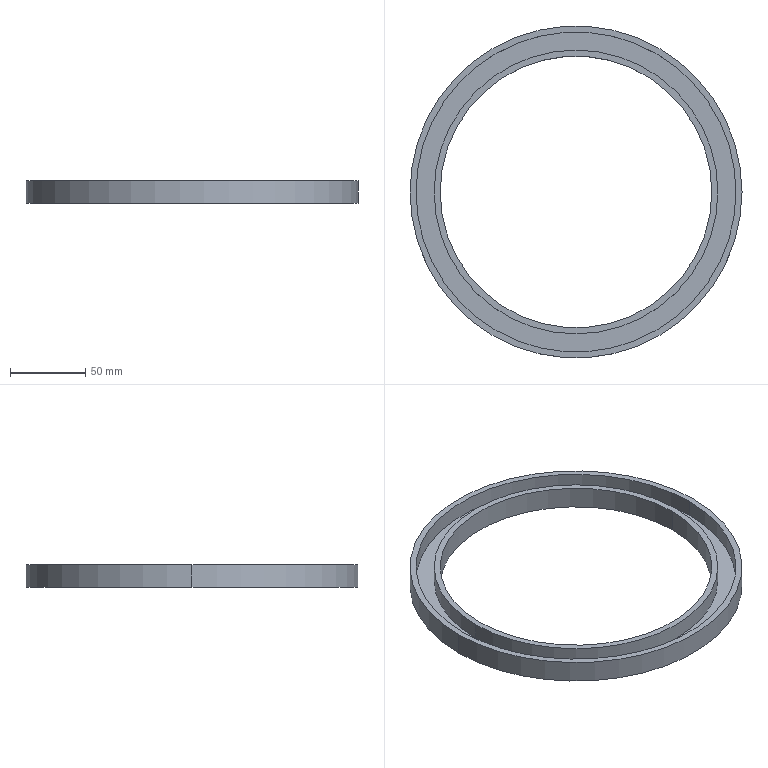Part | SolidWorks | features Extrusion 1, Shell 1 | 1 solid | 12 faces | box 220 x 220 x 15 mm | volume 105558 mm3 | cylinder 8 | plane 4 | commonest cylinder face diameters 180 x2 188 x2 212 x2 220 x2
STEP:
#1=CARTESIAN_POINT('',(94.,0.,15.));
#2=VERTEX_POINT('',#1);
#3=CARTESIAN_POINT('',(-94.,0.,15.));
#4=VERTEX_POINT('',#3);
#5=CARTESIAN_POINT('',(0.,0.,15.));
#6=DIRECTION('',(0.,0.,1.));
#7=DIRECTION('',(1.,0.,0.));
#8=AXIS2_PLACEMENT_3D('',#5,#6,#7);
#9=CIRCLE('',#8,94.);
#10=EDGE_CURVE('',#2,#4,#9,.T.);
#11=ORIENTED_EDGE('',*,*,#10,.F.);
#12=CARTESIAN_POINT('',(94.,0.,4.));
#13=VERTEX_POINT('',#12);
#14=CARTESIAN_POINT('',(94.,0.,15.));
#15=DIRECTION('',(0.,0.,-1.));
#16=VECTOR('',#15,1000.);
#17=LINE('',#14,#16);
#18=EDGE_CURVE('',#2,#13,#17,.T.);
#19=ORIENTED_EDGE('',*,*,#18,.T.);
#20=CARTESIAN_POINT('',(-94.,0.,4.));
#21=VERTEX_POINT('',#20);
#22=CARTESIAN_POINT('',(0.,0.,4.));
#23=DIRECTION('',(0.,0.,1.));
#24=DIRECTION('',(1.,0.,0.));
#25=AXIS2_PLACEMENT_3D('',#22,#23,#24);
#26=CIRCLE('',#25,94.);
#27=EDGE_CURVE('',#13,#21,#26,.T.);
#28=ORIENTED_EDGE('',*,*,#27,.T.);
#29=CARTESIAN_POINT('',(-94.,0.,15.));
#30=DIRECTION('',(0.,0.,-1.));
#31=VECTOR('',#30,1000.);
#32=LINE('',#29,#31);
#33=EDGE_CURVE('',#4,#21,#32,.T.);
#34=ORIENTED_EDGE('',*,*,#33,.F.);
#35=EDGE_LOOP('',(#11,#19,#28,#34));
#36=FACE_OUTER_BOUND('',#35,.T.);
#37=CARTESIAN_POINT('',(0.,0.,15.));
#38=DIRECTION('',(0.,0.,-1.));
#39=DIRECTION('',(-1.,0.,0.));
#40=AXIS2_PLACEMENT_3D('',#37,#38,#39);
#41=CYLINDRICAL_SURFACE('',#40,94.);
#42=ADVANCED_FACE('',(#36),#41,.T.);
#43=CARTESIAN_POINT('',(-106.,0.,15.));
#44=VERTEX_POINT('',#43);
#45=CARTESIAN_POINT('',(106.,0.,15.));
#46=VERTEX_POINT('',#45);
#47=CARTESIAN_POINT('',(0.,0.,15.));
#48=DIRECTION('',(0.,0.,1.));
#49=DIRECTION('',(1.,0.,0.));
#50=AXIS2_PLACEMENT_3D('',#47,#48,#49);
#51=CIRCLE('',#50,106.);
#52=EDGE_CURVE('',#44,#46,#51,.T.);
#53=ORIENTED_EDGE('',*,*,#52,.T.);
#54=CARTESIAN_POINT('',(106.,0.,4.));
#55=VERTEX_POINT('',#54);
#56=CARTESIAN_POINT('',(106.,0.,15.));
#57=DIRECTION('',(0.,0.,-1.));
#58=VECTOR('',#57,1000.);
#59=LINE('',#56,#58);
#60=EDGE_CURVE('',#46,#55,#59,.T.);
#61=ORIENTED_EDGE('',*,*,#60,.T.);
#62=CARTESIAN_POINT('',(-106.,0.,4.));
#63=VERTEX_POINT('',#62);
#64=CARTESIAN_POINT('',(0.,0.,4.));
#65=DIRECTION('',(0.,0.,1.));
#66=DIRECTION('',(1.,0.,0.));
#67=AXIS2_PLACEMENT_3D('',#64,#65,#66);
#68=CIRCLE('',#67,106.);
#69=EDGE_CURVE('',#63,#55,#68,.T.);
#70=ORIENTED_EDGE('',*,*,#69,.F.);
#71=CARTESIAN_POINT('',(-106.,0.,15.));
#72=DIRECTION('',(0.,0.,-1.));
#73=VECTOR('',#72,1000.);
#74=LINE('',#71,#73);
#75=EDGE_CURVE('',#44,#63,#74,.T.);
#76=ORIENTED_EDGE('',*,*,#75,.F.);
#77=EDGE_LOOP('',(#53,#61,#70,#76));
#78=FACE_OUTER_BOUND('',#77,.T.);
#79=CARTESIAN_POINT('',(0.,0.,15.));
#80=DIRECTION('',(0.,0.,-1.));
#81=DIRECTION('',(-1.,0.,0.));
#82=AXIS2_PLACEMENT_3D('',#79,#80,#81);
#83=CYLINDRICAL_SURFACE('',#82,106.);
#84=ADVANCED_FACE('',(#78),#83,.F.);
#85=CARTESIAN_POINT('',(-90.,0.,15.));
#86=VERTEX_POINT('',#85);
#87=CARTESIAN_POINT('',(90.,0.,15.));
#88=VERTEX_POINT('',#87);
#89=CARTESIAN_POINT('',(0.,0.,15.));
#90=DIRECTION('',(0.,0.,1.));
#91=DIRECTION('',(1.,0.,0.));
#92=AXIS2_PLACEMENT_3D('',#89,#90,#91);
#93=CIRCLE('',#92,90.);
#94=EDGE_CURVE('',#86,#88,#93,.T.);
#95=ORIENTED_EDGE('',*,*,#94,.T.);
#96=CARTESIAN_POINT('',(90.,0.,0.));
#97=VERTEX_POINT('',#96);
#98=CARTESIAN_POINT('',(90.,0.,15.));
#99=DIRECTION('',(0.,0.,-1.));
#100=VECTOR('',#99,1000.);
#101=LINE('',#98,#100);
#102=EDGE_CURVE('',#88,#97,#101,.T.);
#103=ORIENTED_EDGE('',*,*,#102,.T.);
#104=CARTESIAN_POINT('',(-90.,0.,0.));
#105=VERTEX_POINT('',#104);
#106=CARTESIAN_POINT('',(0.,0.,0.));
#107=DIRECTION('',(0.,0.,1.));
#108=DIRECTION('',(1.,0.,0.));
#109=AXIS2_PLACEMENT_3D('',#106,#107,#108);
#110=CIRCLE('',#109,90.);
#111=EDGE_CURVE('',#105,#97,#110,.T.);
#112=ORIENTED_EDGE('',*,*,#111,.F.);
#113=CARTESIAN_POINT('',(-90.,0.,15.));
#114=DIRECTION('',(0.,0.,-1.));
#115=VECTOR('',#114,1000.);
#116=LINE('',#113,#115);
#117=EDGE_CURVE('',#86,#105,#116,.T.);
#118=ORIENTED_EDGE('',*,*,#117,.F.);
#119=EDGE_LOOP('',(#95,#103,#112,#118));
#120=FACE_OUTER_BOUND('',#119,.T.);
#121=CARTESIAN_POINT('',(0.,0.,15.));
#122=DIRECTION('',(0.,0.,-1.));
#123=DIRECTION('',(-1.,0.,0.));
#124=AXIS2_PLACEMENT_3D('',#121,#122,#123);
#125=CYLINDRICAL_SURFACE('',#124,90.);
#126=ADVANCED_FACE('',(#120),#125,.F.);
#127=CARTESIAN_POINT('',(110.,0.,15.));
#128=VERTEX_POINT('',#127);
#129=CARTESIAN_POINT('',(-110.,0.,15.));
#130=VERTEX_POINT('',#129);
#131=CARTESIAN_POINT('',(0.,0.,15.));
#132=DIRECTION('',(0.,0.,1.));
#133=DIRECTION('',(1.,0.,0.));
#134=AXIS2_PLACEMENT_3D('',#131,#132,#133);
#135=CIRCLE('',#134,110.);
#136=EDGE_CURVE('',#128,#130,#135,.T.);
#137=ORIENTED_EDGE('',*,*,#136,.F.);
#138=CARTESIAN_POINT('',(110.,0.,0.));
#139=VERTEX_POINT('',#138);
#140=CARTESIAN_POINT('',(110.,0.,15.));
#141=DIRECTION('',(0.,0.,-1.));
#142=VECTOR('',#141,1000.);
#143=LINE('',#140,#142);
#144=EDGE_CURVE('',#128,#139,#143,.T.);
#145=ORIENTED_EDGE('',*,*,#144,.T.);
#146=CARTESIAN_POINT('',(-110.,0.,0.));
#147=VERTEX_POINT('',#146);
#148=CARTESIAN_POINT('',(0.,0.,0.));
#149=DIRECTION('',(0.,0.,1.));
#150=DIRECTION('',(1.,0.,0.));
#151=AXIS2_PLACEMENT_3D('',#148,#149,#150);
#152=CIRCLE('',#151,110.);
#153=EDGE_CURVE('',#139,#147,#152,.T.);
#154=ORIENTED_EDGE('',*,*,#153,.T.);
#155=CARTESIAN_POINT('',(-110.,0.,15.));
#156=DIRECTION('',(0.,0.,-1.));
#157=VECTOR('',#156,1000.);
#158=LINE('',#155,#157);
#159=EDGE_CURVE('',#130,#147,#158,.T.);
#160=ORIENTED_EDGE('',*,*,#159,.F.);
#161=EDGE_LOOP('',(#137,#145,#154,#160));
#162=FACE_OUTER_BOUND('',#161,.T.);
#163=CARTESIAN_POINT('',(0.,0.,15.));
#164=DIRECTION('',(0.,0.,-1.));
#165=DIRECTION('',(-1.,0.,0.));
#166=AXIS2_PLACEMENT_3D('',#163,#164,#165);
#167=CYLINDRICAL_SURFACE('',#166,110.);
#168=ADVANCED_FACE('',(#162),#167,.T.);
#169=ORIENTED_EDGE('',*,*,#94,.F.);
#170=CARTESIAN_POINT('',(0.,0.,15.));
#171=DIRECTION('',(0.,0.,1.));
#172=DIRECTION('',(1.,0.,0.));
#173=AXIS2_PLACEMENT_3D('',#170,#171,#172);
#174=CIRCLE('',#173,90.);
#175=EDGE_CURVE('',#88,#86,#174,.T.);
#176=ORIENTED_EDGE('',*,*,#175,.F.);
#177=EDGE_LOOP('',(#169,#176));
#178=FACE_BOUND('',#177,.T.);
#179=CARTESIAN_POINT('',(0.,0.,15.));
#180=DIRECTION('',(0.,0.,1.));
#181=DIRECTION('',(1.,0.,0.));
#182=AXIS2_PLACEMENT_3D('',#179,#180,#181);
#183=CIRCLE('',#182,94.);
#184=EDGE_CURVE('',#4,#2,#183,.T.);
#185=ORIENTED_EDGE('',*,*,#184,.T.);
#186=ORIENTED_EDGE('',*,*,#10,.T.);
#187=EDGE_LOOP('',(#185,#186));
#188=FACE_OUTER_BOUND('',#187,.T.);
#189=CARTESIAN_POINT('',(0.,0.,15.));
#190=DIRECTION('',(0.,0.,1.));
#191=DIRECTION('',(1.,0.,0.));
#192=AXIS2_PLACEMENT_3D('',#189,#190,#191);
#193=PLANE('',#192);
#194=ADVANCED_FACE('',(#178,#188),#193,.T.);
#195=ORIENTED_EDGE('',*,*,#52,.F.);
#196=CARTESIAN_POINT('',(0.,0.,15.));
#197=DIRECTION('',(0.,0.,1.));
#198=DIRECTION('',(1.,0.,0.));
#199=AXIS2_PLACEMENT_3D('',#196,#197,#198);
#200=CIRCLE('',#199,106.);
#201=EDGE_CURVE('',#46,#44,#200,.T.);
#202=ORIENTED_EDGE('',*,*,#201,.F.);
#203=EDGE_LOOP('',(#195,#202));
#204=FACE_BOUND('',#203,.T.);
#205=CARTESIAN_POINT('',(0.,0.,15.));
#206=DIRECTION('',(0.,0.,1.));
#207=DIRECTION('',(1.,0.,0.));
#208=AXIS2_PLACEMENT_3D('',#205,#206,#207);
#209=CIRCLE('',#208,110.);
#210=EDGE_CURVE('',#130,#128,#209,.T.);
#211=ORIENTED_EDGE('',*,*,#210,.T.);
#212=ORIENTED_EDGE('',*,*,#136,.T.);
#213=EDGE_LOOP('',(#211,#212));
#214=FACE_OUTER_BOUND('',#213,.T.);
#215=CARTESIAN_POINT('',(0.,0.,15.));
#216=DIRECTION('',(0.,0.,1.));
#217=DIRECTION('',(1.,0.,0.));
#218=AXIS2_PLACEMENT_3D('',#215,#216,#217);
#219=PLANE('',#218);
#220=ADVANCED_FACE('',(#204,#214),#219,.T.);
#221=CARTESIAN_POINT('',(0.,0.,0.));
#222=DIRECTION('',(0.,0.,1.));
#223=DIRECTION('',(1.,0.,0.));
#224=AXIS2_PLACEMENT_3D('',#221,#222,#223);
#225=CIRCLE('',#224,110.);
#226=EDGE_CURVE('',#147,#139,#225,.T.);
#227=ORIENTED_EDGE('',*,*,#226,.F.);
#228=ORIENTED_EDGE('',*,*,#153,.F.);
#229=EDGE_LOOP('',(#227,#228));
#230=FACE_OUTER_BOUND('',#229,.T.);
#231=ORIENTED_EDGE('',*,*,#111,.T.);
#232=CARTESIAN_POINT('',(0.,0.,0.));
#233=DIRECTION('',(0.,0.,1.));
#234=DIRECTION('',(1.,0.,0.));
#235=AXIS2_PLACEMENT_3D('',#232,#233,#234);
#236=CIRCLE('',#235,90.);
#237=EDGE_CURVE('',#97,#105,#236,.T.);
#238=ORIENTED_EDGE('',*,*,#237,.T.);
#239=EDGE_LOOP('',(#231,#238));
#240=FACE_BOUND('',#239,.T.);
#241=CARTESIAN_POINT('',(0.,0.,0.));
#242=DIRECTION('',(0.,0.,1.));
#243=DIRECTION('',(1.,0.,0.));
#244=AXIS2_PLACEMENT_3D('',#241,#242,#243);
#245=PLANE('',#244);
#246=ADVANCED_FACE('',(#230,#240),#245,.F.);
#247=ORIENTED_EDGE('',*,*,#144,.F.);
#248=ORIENTED_EDGE('',*,*,#210,.F.);
#249=ORIENTED_EDGE('',*,*,#159,.T.);
#250=ORIENTED_EDGE('',*,*,#226,.T.);
#251=EDGE_LOOP('',(#247,#248,#249,#250));
#252=FACE_OUTER_BOUND('',#251,.T.);
#253=CARTESIAN_POINT('',(0.,0.,15.));
#254=DIRECTION('',(0.,0.,-1.));
#255=DIRECTION('',(-1.,0.,0.));
#256=AXIS2_PLACEMENT_3D('',#253,#254,#255);
#257=CYLINDRICAL_SURFACE('',#256,110.);
#258=ADVANCED_FACE('',(#252),#257,.T.);
#259=ORIENTED_EDGE('',*,*,#102,.F.);
#260=ORIENTED_EDGE('',*,*,#175,.T.);
#261=ORIENTED_EDGE('',*,*,#117,.T.);
#262=ORIENTED_EDGE('',*,*,#237,.F.);
#263=EDGE_LOOP('',(#259,#260,#261,#262));
#264=FACE_OUTER_BOUND('',#263,.T.);
#265=CARTESIAN_POINT('',(0.,0.,15.));
#266=DIRECTION('',(0.,0.,-1.));
#267=DIRECTION('',(-1.,0.,0.));
#268=AXIS2_PLACEMENT_3D('',#265,#266,#267);
#269=CYLINDRICAL_SURFACE('',#268,90.);
#270=ADVANCED_FACE('',(#264),#269,.F.);
#271=ORIENTED_EDGE('',*,*,#69,.T.);
#272=CARTESIAN_POINT('',(0.,0.,4.));
#273=DIRECTION('',(0.,0.,1.));
#274=DIRECTION('',(1.,0.,0.));
#275=AXIS2_PLACEMENT_3D('',#272,#273,#274);
#276=CIRCLE('',#275,106.);
#277=EDGE_CURVE('',#55,#63,#276,.T.);
#278=ORIENTED_EDGE('',*,*,#277,.T.);
#279=EDGE_LOOP('',(#271,#278));
#280=FACE_OUTER_BOUND('',#279,.T.);
#281=CARTESIAN_POINT('',(0.,0.,4.));
#282=DIRECTION('',(0.,0.,1.));
#283=DIRECTION('',(1.,0.,0.));
#284=AXIS2_PLACEMENT_3D('',#281,#282,#283);
#285=CIRCLE('',#284,94.);
#286=EDGE_CURVE('',#21,#13,#285,.T.);
#287=ORIENTED_EDGE('',*,*,#286,.F.);
#288=ORIENTED_EDGE('',*,*,#27,.F.);
#289=EDGE_LOOP('',(#287,#288));
#290=FACE_BOUND('',#289,.T.);
#291=CARTESIAN_POINT('',(0.,0.,4.));
#292=DIRECTION('',(0.,0.,1.));
#293=DIRECTION('',(1.,0.,0.));
#294=AXIS2_PLACEMENT_3D('',#291,#292,#293);
#295=PLANE('',#294);
#296=ADVANCED_FACE('',(#280,#290),#295,.T.);
#297=ORIENTED_EDGE('',*,*,#60,.F.);
#298=ORIENTED_EDGE('',*,*,#201,.T.);
#299=ORIENTED_EDGE('',*,*,#75,.T.);
#300=ORIENTED_EDGE('',*,*,#277,.F.);
#301=EDGE_LOOP('',(#297,#298,#299,#300));
#302=FACE_OUTER_BOUND('',#301,.T.);
#303=CARTESIAN_POINT('',(0.,0.,15.));
#304=DIRECTION('',(0.,0.,-1.));
#305=DIRECTION('',(-1.,0.,0.));
#306=AXIS2_PLACEMENT_3D('',#303,#304,#305);
#307=CYLINDRICAL_SURFACE('',#306,106.);
#308=ADVANCED_FACE('',(#302),#307,.F.);
#309=ORIENTED_EDGE('',*,*,#18,.F.);
#310=ORIENTED_EDGE('',*,*,#184,.F.);
#311=ORIENTED_EDGE('',*,*,#33,.T.);
#312=ORIENTED_EDGE('',*,*,#286,.T.);
#313=EDGE_LOOP('',(#309,#310,#311,#312));
#314=FACE_OUTER_BOUND('',#313,.T.);
#315=CARTESIAN_POINT('',(0.,0.,15.));
#316=DIRECTION('',(0.,0.,-1.));
#317=DIRECTION('',(-1.,0.,0.));
#318=AXIS2_PLACEMENT_3D('',#315,#316,#317);
#319=CYLINDRICAL_SURFACE('',#318,94.);
#320=ADVANCED_FACE('',(#314),#319,.T.);
#321=CLOSED_SHELL('',(#42,#84,#126,#168,#194,#220,#246,#258,#270,#296,#308,#320));
#322=MANIFOLD_SOLID_BREP('',#321);
#323=CARTESIAN_POINT('',(0.,0.,0.));
#324=DIRECTION('',(0.,0.,1.));
#325=DIRECTION('',(1.,0.,0.));
#326=AXIS2_PLACEMENT_3D('',#323,#324,#325);
#327=(LENGTH_UNIT()NAMED_UNIT(*)SI_UNIT(.MILLI.,.METRE.));
#328=UNCERTAINTY_MEASURE_WITH_UNIT(LENGTH_MEASURE(0.00001),#327,'','');
#329=(NAMED_UNIT(*)PLANE_ANGLE_UNIT()SI_UNIT($,.RADIAN.));
#330=(NAMED_UNIT(*)SI_UNIT($,.STERADIAN.)SOLID_ANGLE_UNIT());
#331=(GEOMETRIC_REPRESENTATION_CONTEXT(3)GLOBAL_UNCERTAINTY_ASSIGNED_CONTEXT((#328))GLOBAL_UNIT_ASSIGNED_CONTEXT((#327,#329,#330))REPRESENTATION_CONTEXT('',''));
#332=ADVANCED_BREP_SHAPE_REPRESENTATION('',(#322,#326),#331);